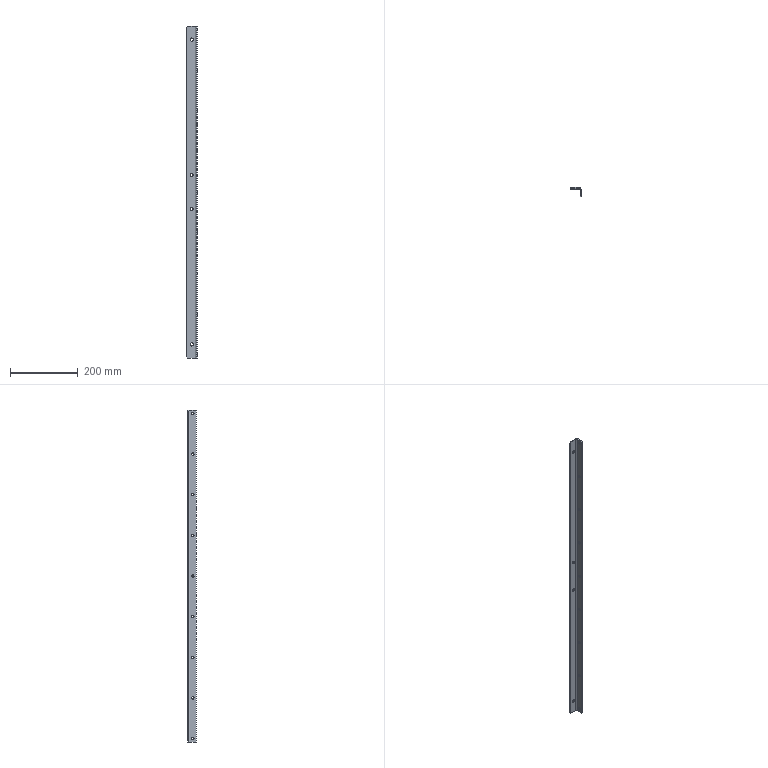Part | NX | features solid 2 | 1 solid | 38 faces | box 30 x 25 x 980 mm | volume 145338 mm3 | cylinder 28 | plane 10 | commonest cylinder face diameters 7 x18 9.2 x8 6 x1 12 x1
STEP:
#1=CARTESIAN_POINT('',(553.,497.,1245.));
#2=VERTEX_POINT('',#1);
#3=CARTESIAN_POINT('',(550.,497.,1242.));
#4=VERTEX_POINT('',#3);
#5=CARTESIAN_POINT('',(550.,497.,1242.));
#6=DIRECTION('',(-0.7071,0.,-0.7071));
#7=VECTOR('',#6,1000.);
#8=LINE('',#5,#7);
#9=EDGE_CURVE('',#2,#4,#8,.T.);
#10=ORIENTED_EDGE('',*,*,#9,.F.);
#11=CARTESIAN_POINT('',(553.,500.,1245.));
#12=VERTEX_POINT('',#11);
#13=CARTESIAN_POINT('',(553.,500.,1245.));
#14=DIRECTION('',(0.,-1.,0.));
#15=VECTOR('',#14,1000.);
#16=LINE('',#13,#15);
#17=EDGE_CURVE('',#12,#2,#16,.T.);
#18=ORIENTED_EDGE('',*,*,#17,.F.);
#19=CARTESIAN_POINT('',(550.,500.,1242.));
#20=VERTEX_POINT('',#19);
#21=CARTESIAN_POINT('',(566.5,500.,1258.5));
#22=DIRECTION('',(0.7071,0.,0.7071));
#23=VECTOR('',#22,1000.);
#24=LINE('',#21,#23);
#25=EDGE_CURVE('',#20,#12,#24,.T.);
#26=ORIENTED_EDGE('',*,*,#25,.F.);
#27=CARTESIAN_POINT('',(550.,500.,1242.));
#28=DIRECTION('',(0.,1.,0.));
#29=VECTOR('',#28,1000.);
#30=LINE('',#27,#29);
#31=EDGE_CURVE('',#4,#20,#30,.T.);
#32=ORIENTED_EDGE('',*,*,#31,.F.);
#33=EDGE_LOOP('',(#10,#18,#26,#32));
#34=FACE_BOUND('',#33,.T.);
#35=CARTESIAN_POINT('',(550.,500.,1242.));
#36=DIRECTION('',(0.7071,0.,-0.7071));
#37=DIRECTION('',(0.,-1.,0.));
#38=AXIS2_PLACEMENT_3D('',#35,#36,#37);
#39=PLANE('',#38);
#40=ADVANCED_FACE('',(#34),#39,.F.);
#41=CARTESIAN_POINT('',(550.,497.,268.));
#42=VERTEX_POINT('',#41);
#43=CARTESIAN_POINT('',(553.,497.,265.));
#44=VERTEX_POINT('',#43);
#45=CARTESIAN_POINT('',(553.,497.,265.));
#46=DIRECTION('',(0.7071,0.,-0.7071));
#47=VECTOR('',#46,1000.);
#48=LINE('',#45,#47);
#49=EDGE_CURVE('',#42,#44,#48,.T.);
#50=ORIENTED_EDGE('',*,*,#49,.F.);
#51=CARTESIAN_POINT('',(550.,500.,268.));
#52=VERTEX_POINT('',#51);
#53=CARTESIAN_POINT('',(550.,500.,268.));
#54=DIRECTION('',(0.,-1.,0.));
#55=VECTOR('',#54,1000.);
#56=LINE('',#53,#55);
#57=EDGE_CURVE('',#52,#42,#56,.T.);
#58=ORIENTED_EDGE('',*,*,#57,.F.);
#59=CARTESIAN_POINT('',(553.,500.,265.));
#60=VERTEX_POINT('',#59);
#61=CARTESIAN_POINT('',(76.5,500.,741.5));
#62=DIRECTION('',(-0.7071,0.,0.7071));
#63=VECTOR('',#62,1000.);
#64=LINE('',#61,#63);
#65=EDGE_CURVE('',#60,#52,#64,.T.);
#66=ORIENTED_EDGE('',*,*,#65,.F.);
#67=CARTESIAN_POINT('',(553.,500.,265.));
#68=DIRECTION('',(0.,1.,0.));
#69=VECTOR('',#68,1000.);
#70=LINE('',#67,#69);
#71=EDGE_CURVE('',#44,#60,#70,.T.);
#72=ORIENTED_EDGE('',*,*,#71,.F.);
#73=EDGE_LOOP('',(#50,#58,#66,#72));
#74=FACE_BOUND('',#73,.T.);
#75=CARTESIAN_POINT('',(553.,500.,265.));
#76=DIRECTION('',(-0.7071,0.,-0.7071));
#77=DIRECTION('',(-0.7071,0.,0.7071));
#78=AXIS2_PLACEMENT_3D('',#75,#76,#77);
#79=PLANE('',#78);
#80=ADVANCED_FACE('',(#74),#79,.T.);
#81=CARTESIAN_POINT('',(577.,488.5,1235.));
#82=VERTEX_POINT('',#81);
#83=CARTESIAN_POINT('',(580.,488.5,1235.));
#84=VERTEX_POINT('',#83);
#85=CARTESIAN_POINT('',(1557.778,488.5,1235.));
#86=DIRECTION('',(-1.,0.,0.));
#87=VECTOR('',#86,1000.);
#88=LINE('',#85,#87);
#89=EDGE_CURVE('',#82,#84,#88,.F.);
#90=ORIENTED_EDGE('',*,*,#89,.T.);
#91=CARTESIAN_POINT('',(580.,481.5,1235.));
#92=VERTEX_POINT('',#91);
#93=CARTESIAN_POINT('',(580.,485.,1235.));
#94=DIRECTION('',(-1.,0.,0.));
#95=DIRECTION('',(0.,-1.,0.));
#96=AXIS2_PLACEMENT_3D('',#93,#94,#95);
#97=CIRCLE('',#96,3.5);
#98=EDGE_CURVE('',#92,#84,#97,.T.);
#99=ORIENTED_EDGE('',*,*,#98,.F.);
#100=CARTESIAN_POINT('',(577.,481.5,1235.));
#101=VERTEX_POINT('',#100);
#102=CARTESIAN_POINT('',(1557.778,481.5,1235.));
#103=DIRECTION('',(-1.,0.,0.));
#104=VECTOR('',#103,1000.);
#105=LINE('',#102,#104);
#106=EDGE_CURVE('',#92,#101,#105,.T.);
#107=ORIENTED_EDGE('',*,*,#106,.T.);
#108=CARTESIAN_POINT('',(577.,485.,1235.));
#109=DIRECTION('',(-1.,0.,0.));
#110=DIRECTION('',(0.,0.,-1.));
#111=AXIS2_PLACEMENT_3D('',#108,#109,#110);
#112=CIRCLE('',#111,3.5);
#113=EDGE_CURVE('',#101,#82,#112,.T.);
#114=ORIENTED_EDGE('',*,*,#113,.T.);
#115=EDGE_LOOP('',(#90,#99,#107,#114));
#116=FACE_BOUND('',#115,.T.);
#117=CARTESIAN_POINT('',(1557.778,485.,1235.));
#118=DIRECTION('',(-1.,0.,0.));
#119=DIRECTION('',(0.,-1.,0.));
#120=AXIS2_PLACEMENT_3D('',#117,#118,#119);
#121=CYLINDRICAL_SURFACE('',#120,3.5);
#122=ADVANCED_FACE('',(#116),#121,.F.);
#123=CARTESIAN_POINT('',(580.,488.5,275.));
#124=VERTEX_POINT('',#123);
#125=CARTESIAN_POINT('',(577.,488.5,275.));
#126=VERTEX_POINT('',#125);
#127=CARTESIAN_POINT('',(1557.778,488.5,275.));
#128=DIRECTION('',(-1.,0.,0.));
#129=VECTOR('',#128,1000.);
#130=LINE('',#127,#129);
#131=EDGE_CURVE('',#124,#126,#130,.T.);
#132=ORIENTED_EDGE('',*,*,#131,.F.);
#133=CARTESIAN_POINT('',(580.,481.5,275.));
#134=VERTEX_POINT('',#133);
#135=CARTESIAN_POINT('',(580.,485.,275.));
#136=DIRECTION('',(-1.,0.,0.));
#137=DIRECTION('',(0.,-1.,0.));
#138=AXIS2_PLACEMENT_3D('',#135,#136,#137);
#139=CIRCLE('',#138,3.5);
#140=EDGE_CURVE('',#134,#124,#139,.T.);
#141=ORIENTED_EDGE('',*,*,#140,.F.);
#142=CARTESIAN_POINT('',(577.,481.5,275.));
#143=VERTEX_POINT('',#142);
#144=CARTESIAN_POINT('',(1557.778,481.5,275.));
#145=DIRECTION('',(-1.,0.,0.));
#146=VECTOR('',#145,1000.);
#147=LINE('',#144,#146);
#148=EDGE_CURVE('',#143,#134,#147,.F.);
#149=ORIENTED_EDGE('',*,*,#148,.F.);
#150=CARTESIAN_POINT('',(577.,485.,275.));
#151=DIRECTION('',(-1.,0.,0.));
#152=DIRECTION('',(0.,0.,-1.));
#153=AXIS2_PLACEMENT_3D('',#150,#151,#152);
#154=CIRCLE('',#153,3.5);
#155=EDGE_CURVE('',#143,#126,#154,.T.);
#156=ORIENTED_EDGE('',*,*,#155,.T.);
#157=EDGE_LOOP('',(#132,#141,#149,#156));
#158=FACE_BOUND('',#157,.T.);
#159=CARTESIAN_POINT('',(1557.778,485.,275.));
#160=DIRECTION('',(-1.,0.,0.));
#161=DIRECTION('',(0.,-1.,0.));
#162=AXIS2_PLACEMENT_3D('',#159,#160,#161);
#163=CYLINDRICAL_SURFACE('',#162,3.5);
#164=ADVANCED_FACE('',(#158),#163,.F.);
#165=CARTESIAN_POINT('',(580.,488.5,395.));
#166=VERTEX_POINT('',#165);
#167=CARTESIAN_POINT('',(577.,488.5,395.));
#168=VERTEX_POINT('',#167);
#169=CARTESIAN_POINT('',(1557.778,488.5,395.));
#170=DIRECTION('',(-1.,0.,0.));
#171=VECTOR('',#170,1000.);
#172=LINE('',#169,#171);
#173=EDGE_CURVE('',#166,#168,#172,.T.);
#174=ORIENTED_EDGE('',*,*,#173,.F.);
#175=CARTESIAN_POINT('',(580.,481.5,395.));
#176=VERTEX_POINT('',#175);
#177=CARTESIAN_POINT('',(580.,485.,395.));
#178=DIRECTION('',(-1.,0.,0.));
#179=DIRECTION('',(0.,-1.,0.));
#180=AXIS2_PLACEMENT_3D('',#177,#178,#179);
#181=CIRCLE('',#180,3.5);
#182=EDGE_CURVE('',#176,#166,#181,.T.);
#183=ORIENTED_EDGE('',*,*,#182,.F.);
#184=CARTESIAN_POINT('',(577.,481.5,395.));
#185=VERTEX_POINT('',#184);
#186=CARTESIAN_POINT('',(1557.778,481.5,395.));
#187=DIRECTION('',(-1.,0.,0.));
#188=VECTOR('',#187,1000.);
#189=LINE('',#186,#188);
#190=EDGE_CURVE('',#185,#176,#189,.F.);
#191=ORIENTED_EDGE('',*,*,#190,.F.);
#192=CARTESIAN_POINT('',(577.,485.,395.));
#193=DIRECTION('',(-1.,0.,0.));
#194=DIRECTION('',(0.,0.,-1.));
#195=AXIS2_PLACEMENT_3D('',#192,#193,#194);
#196=CIRCLE('',#195,3.5);
#197=EDGE_CURVE('',#185,#168,#196,.T.);
#198=ORIENTED_EDGE('',*,*,#197,.T.);
#199=EDGE_LOOP('',(#174,#183,#191,#198));
#200=FACE_BOUND('',#199,.T.);
#201=CARTESIAN_POINT('',(1557.778,485.,395.));
#202=DIRECTION('',(-1.,0.,0.));
#203=DIRECTION('',(0.,-1.,0.));
#204=AXIS2_PLACEMENT_3D('',#201,#202,#203);
#205=CYLINDRICAL_SURFACE('',#204,3.5);
#206=ADVANCED_FACE('',(#200),#205,.F.);
#207=CARTESIAN_POINT('',(577.,488.5,1115.));
#208=VERTEX_POINT('',#207);
#209=CARTESIAN_POINT('',(580.,488.5,1115.));
#210=VERTEX_POINT('',#209);
#211=CARTESIAN_POINT('',(1557.778,488.5,1115.));
#212=DIRECTION('',(-1.,0.,0.));
#213=VECTOR('',#212,1000.);
#214=LINE('',#211,#213);
#215=EDGE_CURVE('',#208,#210,#214,.F.);
#216=ORIENTED_EDGE('',*,*,#215,.T.);
#217=CARTESIAN_POINT('',(580.,481.5,1115.));
#218=VERTEX_POINT('',#217);
#219=CARTESIAN_POINT('',(580.,485.,1115.));
#220=DIRECTION('',(-1.,0.,0.));
#221=DIRECTION('',(0.,-1.,0.));
#222=AXIS2_PLACEMENT_3D('',#219,#220,#221);
#223=CIRCLE('',#222,3.5);
#224=EDGE_CURVE('',#218,#210,#223,.T.);
#225=ORIENTED_EDGE('',*,*,#224,.F.);
#226=CARTESIAN_POINT('',(577.,481.5,1115.));
#227=VERTEX_POINT('',#226);
#228=CARTESIAN_POINT('',(1557.778,481.5,1115.));
#229=DIRECTION('',(-1.,0.,0.));
#230=VECTOR('',#229,1000.);
#231=LINE('',#228,#230);
#232=EDGE_CURVE('',#218,#227,#231,.T.);
#233=ORIENTED_EDGE('',*,*,#232,.T.);
#234=CARTESIAN_POINT('',(577.,485.,1115.));
#235=DIRECTION('',(-1.,0.,0.));
#236=DIRECTION('',(0.,0.,-1.));
#237=AXIS2_PLACEMENT_3D('',#234,#235,#236);
#238=CIRCLE('',#237,3.5);
#239=EDGE_CURVE('',#227,#208,#238,.T.);
#240=ORIENTED_EDGE('',*,*,#239,.T.);
#241=EDGE_LOOP('',(#216,#225,#233,#240));
#242=FACE_BOUND('',#241,.T.);
#243=CARTESIAN_POINT('',(1557.778,485.,1115.));
#244=DIRECTION('',(-1.,0.,0.));
#245=DIRECTION('',(0.,-1.,0.));
#246=AXIS2_PLACEMENT_3D('',#243,#244,#245);
#247=CYLINDRICAL_SURFACE('',#246,3.5);
#248=ADVANCED_FACE('',(#242),#247,.F.);
#249=CARTESIAN_POINT('',(577.,488.5,995.));
#250=VERTEX_POINT('',#249);
#251=CARTESIAN_POINT('',(580.,488.5,995.));
#252=VERTEX_POINT('',#251);
#253=CARTESIAN_POINT('',(1557.778,488.5,995.));
#254=DIRECTION('',(-1.,0.,0.));
#255=VECTOR('',#254,1000.);
#256=LINE('',#253,#255);
#257=EDGE_CURVE('',#250,#252,#256,.F.);
#258=ORIENTED_EDGE('',*,*,#257,.T.);
#259=CARTESIAN_POINT('',(580.,481.5,995.));
#260=VERTEX_POINT('',#259);
#261=CARTESIAN_POINT('',(580.,485.,995.));
#262=DIRECTION('',(-1.,0.,0.));
#263=DIRECTION('',(0.,-1.,0.));
#264=AXIS2_PLACEMENT_3D('',#261,#262,#263);
#265=CIRCLE('',#264,3.5);
#266=EDGE_CURVE('',#260,#252,#265,.T.);
#267=ORIENTED_EDGE('',*,*,#266,.F.);
#268=CARTESIAN_POINT('',(577.,481.5,995.));
#269=VERTEX_POINT('',#268);
#270=CARTESIAN_POINT('',(1557.778,481.5,995.));
#271=DIRECTION('',(-1.,0.,0.));
#272=VECTOR('',#271,1000.);
#273=LINE('',#270,#272);
#274=EDGE_CURVE('',#260,#269,#273,.T.);
#275=ORIENTED_EDGE('',*,*,#274,.T.);
#276=CARTESIAN_POINT('',(577.,485.,995.));
#277=DIRECTION('',(-1.,0.,0.));
#278=DIRECTION('',(0.,0.,-1.));
#279=AXIS2_PLACEMENT_3D('',#276,#277,#278);
#280=CIRCLE('',#279,3.5);
#281=EDGE_CURVE('',#269,#250,#280,.T.);
#282=ORIENTED_EDGE('',*,*,#281,.T.);
#283=EDGE_LOOP('',(#258,#267,#275,#282));
#284=FACE_BOUND('',#283,.T.);
#285=CARTESIAN_POINT('',(1557.778,485.,995.));
#286=DIRECTION('',(-1.,0.,0.));
#287=DIRECTION('',(0.,-1.,0.));
#288=AXIS2_PLACEMENT_3D('',#285,#286,#287);
#289=CYLINDRICAL_SURFACE('',#288,3.5);
#290=ADVANCED_FACE('',(#284),#289,.F.);
#291=CARTESIAN_POINT('',(580.,488.5,875.));
#292=VERTEX_POINT('',#291);
#293=CARTESIAN_POINT('',(577.,488.5,875.));
#294=VERTEX_POINT('',#293);
#295=CARTESIAN_POINT('',(1557.778,488.5,875.));
#296=DIRECTION('',(-1.,0.,0.));
#297=VECTOR('',#296,1000.);
#298=LINE('',#295,#297);
#299=EDGE_CURVE('',#292,#294,#298,.T.);
#300=ORIENTED_EDGE('',*,*,#299,.F.);
#301=CARTESIAN_POINT('',(580.,481.5,875.));
#302=VERTEX_POINT('',#301);
#303=CARTESIAN_POINT('',(580.,485.,875.));
#304=DIRECTION('',(-1.,0.,0.));
#305=DIRECTION('',(0.,-1.,0.));
#306=AXIS2_PLACEMENT_3D('',#303,#304,#305);
#307=CIRCLE('',#306,3.5);
#308=EDGE_CURVE('',#302,#292,#307,.T.);
#309=ORIENTED_EDGE('',*,*,#308,.F.);
#310=CARTESIAN_POINT('',(577.,481.5,875.));
#311=VERTEX_POINT('',#310);
#312=CARTESIAN_POINT('',(1557.778,481.5,875.));
#313=DIRECTION('',(-1.,0.,0.));
#314=VECTOR('',#313,1000.);
#315=LINE('',#312,#314);
#316=EDGE_CURVE('',#311,#302,#315,.F.);
#317=ORIENTED_EDGE('',*,*,#316,.F.);
#318=CARTESIAN_POINT('',(577.,485.,875.));
#319=DIRECTION('',(-1.,0.,0.));
#320=DIRECTION('',(0.,0.,-1.));
#321=AXIS2_PLACEMENT_3D('',#318,#319,#320);
#322=CIRCLE('',#321,3.5);
#323=EDGE_CURVE('',#311,#294,#322,.T.);
#324=ORIENTED_EDGE('',*,*,#323,.T.);
#325=EDGE_LOOP('',(#300,#309,#317,#324));
#326=FACE_BOUND('',#325,.T.);
#327=CARTESIAN_POINT('',(1557.778,485.,875.));
#328=DIRECTION('',(-1.,0.,0.));
#329=DIRECTION('',(0.,-1.,0.));
#330=AXIS2_PLACEMENT_3D('',#327,#328,#329);
#331=CYLINDRICAL_SURFACE('',#330,3.5);
#332=ADVANCED_FACE('',(#326),#331,.F.);
#333=CARTESIAN_POINT('',(580.,488.5,755.));
#334=VERTEX_POINT('',#333);
#335=CARTESIAN_POINT('',(577.,488.5,755.));
#336=VERTEX_POINT('',#335);
#337=CARTESIAN_POINT('',(1557.778,488.5,755.));
#338=DIRECTION('',(-1.,0.,0.));
#339=VECTOR('',#338,1000.);
#340=LINE('',#337,#339);
#341=EDGE_CURVE('',#334,#336,#340,.T.);
#342=ORIENTED_EDGE('',*,*,#341,.F.);
#343=CARTESIAN_POINT('',(580.,481.5,755.));
#344=VERTEX_POINT('',#343);
#345=CARTESIAN_POINT('',(580.,485.,755.));
#346=DIRECTION('',(-1.,0.,0.));
#347=DIRECTION('',(0.,-1.,0.));
#348=AXIS2_PLACEMENT_3D('',#345,#346,#347);
#349=CIRCLE('',#348,3.5);
#350=EDGE_CURVE('',#344,#334,#349,.T.);
#351=ORIENTED_EDGE('',*,*,#350,.F.);
#352=CARTESIAN_POINT('',(577.,481.5,755.));
#353=VERTEX_POINT('',#352);
#354=CARTESIAN_POINT('',(1557.778,481.5,755.));
#355=DIRECTION('',(-1.,0.,0.));
#356=VECTOR('',#355,1000.);
#357=LINE('',#354,#356);
#358=EDGE_CURVE('',#353,#344,#357,.F.);
#359=ORIENTED_EDGE('',*,*,#358,.F.);
#360=CARTESIAN_POINT('',(577.,485.,755.));
#361=DIRECTION('',(-1.,0.,0.));
#362=DIRECTION('',(0.,0.,-1.));
#363=AXIS2_PLACEMENT_3D('',#360,#361,#362);
#364=CIRCLE('',#363,3.5);
#365=EDGE_CURVE('',#353,#336,#364,.T.);
#366=ORIENTED_EDGE('',*,*,#365,.T.);
#367=EDGE_LOOP('',(#342,#351,#359,#366));
#368=FACE_BOUND('',#367,.T.);
#369=CARTESIAN_POINT('',(1557.778,485.,755.));
#370=DIRECTION('',(-1.,0.,0.));
#371=DIRECTION('',(0.,-1.,0.));
#372=AXIS2_PLACEMENT_3D('',#369,#370,#371);
#373=CYLINDRICAL_SURFACE('',#372,3.5);
#374=ADVANCED_FACE('',(#368),#373,.F.);
#375=CARTESIAN_POINT('',(577.,488.5,635.));
#376=VERTEX_POINT('',#375);
#377=CARTESIAN_POINT('',(580.,488.5,635.));
#378=VERTEX_POINT('',#377);
#379=CARTESIAN_POINT('',(1557.778,488.5,635.));
#380=DIRECTION('',(-1.,0.,0.));
#381=VECTOR('',#380,1000.);
#382=LINE('',#379,#381);
#383=EDGE_CURVE('',#376,#378,#382,.F.);
#384=ORIENTED_EDGE('',*,*,#383,.T.);
#385=CARTESIAN_POINT('',(580.,481.5,635.));
#386=VERTEX_POINT('',#385);
#387=CARTESIAN_POINT('',(580.,485.,635.));
#388=DIRECTION('',(-1.,0.,0.));
#389=DIRECTION('',(0.,-1.,0.));
#390=AXIS2_PLACEMENT_3D('',#387,#388,#389);
#391=CIRCLE('',#390,3.5);
#392=EDGE_CURVE('',#386,#378,#391,.T.);
#393=ORIENTED_EDGE('',*,*,#392,.F.);
#394=CARTESIAN_POINT('',(577.,481.5,635.));
#395=VERTEX_POINT('',#394);
#396=CARTESIAN_POINT('',(1557.778,481.5,635.));
#397=DIRECTION('',(-1.,0.,0.));
#398=VECTOR('',#397,1000.);
#399=LINE('',#396,#398);
#400=EDGE_CURVE('',#386,#395,#399,.T.);
#401=ORIENTED_EDGE('',*,*,#400,.T.);
#402=CARTESIAN_POINT('',(577.,485.,635.));
#403=DIRECTION('',(-1.,0.,0.));
#404=DIRECTION('',(0.,0.,-1.));
#405=AXIS2_PLACEMENT_3D('',#402,#403,#404);
#406=CIRCLE('',#405,3.5);
#407=EDGE_CURVE('',#395,#376,#406,.T.);
#408=ORIENTED_EDGE('',*,*,#407,.T.);
#409=EDGE_LOOP('',(#384,#393,#401,#408));
#410=FACE_BOUND('',#409,.T.);
#411=CARTESIAN_POINT('',(1557.778,485.,635.));
#412=DIRECTION('',(-1.,0.,0.));
#413=DIRECTION('',(0.,-1.,0.));
#414=AXIS2_PLACEMENT_3D('',#411,#412,#413);
#415=CYLINDRICAL_SURFACE('',#414,3.5);
#416=ADVANCED_FACE('',(#410),#415,.F.);
#417=CARTESIAN_POINT('',(580.,488.5,515.));
#418=VERTEX_POINT('',#417);
#419=CARTESIAN_POINT('',(577.,488.5,515.));
#420=VERTEX_POINT('',#419);
#421=CARTESIAN_POINT('',(1557.778,488.5,515.));
#422=DIRECTION('',(-1.,0.,0.));
#423=VECTOR('',#422,1000.);
#424=LINE('',#421,#423);
#425=EDGE_CURVE('',#418,#420,#424,.T.);
#426=ORIENTED_EDGE('',*,*,#425,.F.);
#427=CARTESIAN_POINT('',(580.,481.5,515.));
#428=VERTEX_POINT('',#427);
#429=CARTESIAN_POINT('',(580.,485.,515.));
#430=DIRECTION('',(-1.,0.,0.));
#431=DIRECTION('',(0.,-1.,0.));
#432=AXIS2_PLACEMENT_3D('',#429,#430,#431);
#433=CIRCLE('',#432,3.5);
#434=EDGE_CURVE('',#428,#418,#433,.T.);
#435=ORIENTED_EDGE('',*,*,#434,.F.);
#436=CARTESIAN_POINT('',(577.,481.5,515.));
#437=VERTEX_POINT('',#436);
#438=CARTESIAN_POINT('',(1557.778,481.5,515.));
#439=DIRECTION('',(-1.,0.,0.));
#440=VECTOR('',#439,1000.);
#441=LINE('',#438,#440);
#442=EDGE_CURVE('',#437,#428,#441,.F.);
#443=ORIENTED_EDGE('',*,*,#442,.F.);
#444=CARTESIAN_POINT('',(577.,485.,515.));
#445=DIRECTION('',(-1.,0.,0.));
#446=DIRECTION('',(0.,0.,-1.));
#447=AXIS2_PLACEMENT_3D('',#444,#445,#446);
#448=CIRCLE('',#447,3.5);
#449=EDGE_CURVE('',#437,#420,#448,.T.);
#450=ORIENTED_EDGE('',*,*,#449,.T.);
#451=EDGE_LOOP('',(#426,#435,#443,#450));
#452=FACE_BOUND('',#451,.T.);
#453=CARTESIAN_POINT('',(1557.778,485.,515.));
#454=DIRECTION('',(-1.,0.,0.));
#455=DIRECTION('',(0.,-1.,0.));
#456=AXIS2_PLACEMENT_3D('',#453,#454,#455);
#457=CYLINDRICAL_SURFACE('',#456,3.5);
#458=ADVANCED_FACE('',(#452),#457,.F.);
#459=CARTESIAN_POINT('',(564.,500.,1209.6));
#460=VERTEX_POINT('',#459);
#461=CARTESIAN_POINT('',(564.,497.,1209.6));
#462=VERTEX_POINT('',#461);
#463=CARTESIAN_POINT('',(564.,-480.778,1209.6));
#464=DIRECTION('',(0.,1.,0.));
#465=VECTOR('',#464,1000.);
#466=LINE('',#463,#465);
#467=EDGE_CURVE('',#460,#462,#466,.F.);
#468=ORIENTED_EDGE('',*,*,#467,.T.);
#469=CARTESIAN_POINT('',(564.,497.,1200.4));
#470=VERTEX_POINT('',#469);
#471=CARTESIAN_POINT('',(564.,497.,1205.));
#472=DIRECTION('',(0.,1.,0.));
#473=DIRECTION('',(0.,0.,-1.));
#474=AXIS2_PLACEMENT_3D('',#471,#472,#473);
#475=CIRCLE('',#474,4.6);
#476=EDGE_CURVE('',#470,#462,#475,.T.);
#477=ORIENTED_EDGE('',*,*,#476,.F.);
#478=CARTESIAN_POINT('',(564.,500.,1200.4));
#479=VERTEX_POINT('',#478);
#480=CARTESIAN_POINT('',(564.,-480.778,1200.4));
#481=DIRECTION('',(0.,1.,0.));
#482=VECTOR('',#481,1000.);
#483=LINE('',#480,#482);
#484=EDGE_CURVE('',#470,#479,#483,.T.);
#485=ORIENTED_EDGE('',*,*,#484,.T.);
#486=CARTESIAN_POINT('',(564.,500.,1205.));
#487=DIRECTION('',(0.,1.,0.));
#488=DIRECTION('',(0.,0.,1.));
#489=AXIS2_PLACEMENT_3D('',#486,#487,#488);
#490=CIRCLE('',#489,4.6);
#491=EDGE_CURVE('',#479,#460,#490,.T.);
#492=ORIENTED_EDGE('',*,*,#491,.T.);
#493=EDGE_LOOP('',(#468,#477,#485,#492));
#494=FACE_BOUND('',#493,.T.);
#495=CARTESIAN_POINT('',(564.,-480.778,1205.));
#496=DIRECTION('',(0.,1.,0.));
#497=DIRECTION('',(0.,0.,-1.));
#498=AXIS2_PLACEMENT_3D('',#495,#496,#497);
#499=CYLINDRICAL_SURFACE('',#498,4.6);
#500=ADVANCED_FACE('',(#494),#499,.F.);
#501=CARTESIAN_POINT('',(564.,497.,709.6));
#502=VERTEX_POINT('',#501);
#503=CARTESIAN_POINT('',(564.,500.,709.6));
#504=VERTEX_POINT('',#503);
#505=CARTESIAN_POINT('',(564.,-480.778,709.6));
#506=DIRECTION('',(0.,1.,0.));
#507=VECTOR('',#506,1000.);
#508=LINE('',#505,#507);
#509=EDGE_CURVE('',#502,#504,#508,.T.);
#510=ORIENTED_EDGE('',*,*,#509,.F.);
#511=CARTESIAN_POINT('',(564.,497.,700.4));
#512=VERTEX_POINT('',#511);
#513=CARTESIAN_POINT('',(564.,497.,705.));
#514=DIRECTION('',(0.,1.,0.));
#515=DIRECTION('',(0.,0.,-1.));
#516=AXIS2_PLACEMENT_3D('',#513,#514,#515);
#517=CIRCLE('',#516,4.6);
#518=EDGE_CURVE('',#512,#502,#517,.T.);
#519=ORIENTED_EDGE('',*,*,#518,.F.);
#520=CARTESIAN_POINT('',(564.,500.,700.4));
#521=VERTEX_POINT('',#520);
#522=CARTESIAN_POINT('',(564.,-480.778,700.4));
#523=DIRECTION('',(0.,1.,0.));
#524=VECTOR('',#523,1000.);
#525=LINE('',#522,#524);
#526=EDGE_CURVE('',#521,#512,#525,.F.);
#527=ORIENTED_EDGE('',*,*,#526,.F.);
#528=CARTESIAN_POINT('',(564.,500.,705.));
#529=DIRECTION('',(0.,1.,0.));
#530=DIRECTION('',(0.,0.,1.));
#531=AXIS2_PLACEMENT_3D('',#528,#529,#530);
#532=CIRCLE('',#531,4.6);
#533=EDGE_CURVE('',#521,#504,#532,.T.);
#534=ORIENTED_EDGE('',*,*,#533,.T.);
#535=EDGE_LOOP('',(#510,#519,#527,#534));
#536=FACE_BOUND('',#535,.T.);
#537=CARTESIAN_POINT('',(564.,-480.778,705.));
#538=DIRECTION('',(0.,1.,0.));
#539=DIRECTION('',(0.,0.,-1.));
#540=AXIS2_PLACEMENT_3D('',#537,#538,#539);
#541=CYLINDRICAL_SURFACE('',#540,4.6);
#542=ADVANCED_FACE('',(#536),#541,.F.);
#543=CARTESIAN_POINT('',(564.,500.,809.6));
#544=VERTEX_POINT('',#543);
#545=CARTESIAN_POINT('',(564.,497.,809.6));
#546=VERTEX_POINT('',#545);
#547=CARTESIAN_POINT('',(564.,-480.778,809.6));
#548=DIRECTION('',(0.,1.,0.));
#549=VECTOR('',#548,1000.);
#550=LINE('',#547,#549);
#551=EDGE_CURVE('',#544,#546,#550,.F.);
#552=ORIENTED_EDGE('',*,*,#551,.T.);
#553=CARTESIAN_POINT('',(564.,497.,800.4));
#554=VERTEX_POINT('',#553);
#555=CARTESIAN_POINT('',(564.,497.,805.));
#556=DIRECTION('',(0.,1.,0.));
#557=DIRECTION('',(0.,0.,-1.));
#558=AXIS2_PLACEMENT_3D('',#555,#556,#557);
#559=CIRCLE('',#558,4.6);
#560=EDGE_CURVE('',#554,#546,#559,.T.);
#561=ORIENTED_EDGE('',*,*,#560,.F.);
#562=CARTESIAN_POINT('',(564.,500.,800.4));
#563=VERTEX_POINT('',#562);
#564=CARTESIAN_POINT('',(564.,-480.778,800.4));
#565=DIRECTION('',(0.,1.,0.));
#566=VECTOR('',#565,1000.);
#567=LINE('',#564,#566);
#568=EDGE_CURVE('',#554,#563,#567,.T.);
#569=ORIENTED_EDGE('',*,*,#568,.T.);
#570=CARTESIAN_POINT('',(564.,500.,805.));
#571=DIRECTION('',(0.,1.,0.));
#572=DIRECTION('',(0.,0.,1.));
#573=AXIS2_PLACEMENT_3D('',#570,#571,#572);
#574=CIRCLE('',#573,4.6);
#575=EDGE_CURVE('',#563,#544,#574,.T.);
#576=ORIENTED_EDGE('',*,*,#575,.T.);
#577=EDGE_LOOP('',(#552,#561,#569,#576));
#578=FACE_BOUND('',#577,.T.);
#579=CARTESIAN_POINT('',(564.,-480.778,805.));
#580=DIRECTION('',(0.,1.,0.));
#581=DIRECTION('',(0.,0.,-1.));
#582=AXIS2_PLACEMENT_3D('',#579,#580,#581);
#583=CYLINDRICAL_SURFACE('',#582,4.6);
#584=ADVANCED_FACE('',(#578),#583,.F.);
#585=CARTESIAN_POINT('',(564.,500.,309.6));
#586=VERTEX_POINT('',#585);
#587=CARTESIAN_POINT('',(564.,497.,309.6));
#588=VERTEX_POINT('',#587);
#589=CARTESIAN_POINT('',(564.,-480.778,309.6));
#590=DIRECTION('',(0.,1.,0.));
#591=VECTOR('',#590,1000.);
#592=LINE('',#589,#591);
#593=EDGE_CURVE('',#586,#588,#592,.F.);
#594=ORIENTED_EDGE('',*,*,#593,.T.);
#595=CARTESIAN_POINT('',(564.,497.,300.4));
#596=VERTEX_POINT('',#595);
#597=CARTESIAN_POINT('',(564.,497.,305.));
#598=DIRECTION('',(0.,1.,0.));
#599=DIRECTION('',(0.,0.,-1.));
#600=AXIS2_PLACEMENT_3D('',#597,#598,#599);
#601=CIRCLE('',#600,4.6);
#602=EDGE_CURVE('',#596,#588,#601,.T.);
#603=ORIENTED_EDGE('',*,*,#602,.F.);
#604=CARTESIAN_POINT('',(564.,500.,300.4));
#605=VERTEX_POINT('',#604);
#606=CARTESIAN_POINT('',(564.,-480.778,300.4));
#607=DIRECTION('',(0.,1.,0.));
#608=VECTOR('',#607,1000.);
#609=LINE('',#606,#608);
#610=EDGE_CURVE('',#596,#605,#609,.T.);
#611=ORIENTED_EDGE('',*,*,#610,.T.);
#612=CARTESIAN_POINT('',(564.,500.,305.));
#613=DIRECTION('',(0.,1.,0.));
#614=DIRECTION('',(0.,0.,1.));
#615=AXIS2_PLACEMENT_3D('',#612,#613,#614);
#616=CIRCLE('',#615,4.6);
#617=EDGE_CURVE('',#605,#586,#616,.T.);
#618=ORIENTED_EDGE('',*,*,#617,.T.);
#619=EDGE_LOOP('',(#594,#603,#611,#618));
#620=FACE_BOUND('',#619,.T.);
#621=CARTESIAN_POINT('',(564.,-480.778,305.));
#622=DIRECTION('',(0.,1.,0.));
#623=DIRECTION('',(0.,0.,-1.));
#624=AXIS2_PLACEMENT_3D('',#621,#622,#623);
#625=CYLINDRICAL_SURFACE('',#624,4.6);
#626=ADVANCED_FACE('',(#620),#625,.F.);
#627=CARTESIAN_POINT('',(574.,497.,1245.));
#628=VERTEX_POINT('',#627);
#629=CARTESIAN_POINT('',(574.,497.,265.));
#630=VERTEX_POINT('',#629);
#631=CARTESIAN_POINT('',(574.,497.,1245.));
#632=DIRECTION('',(0.,0.,-1.));
#633=VECTOR('',#632,1000.);
#634=LINE('',#631,#633);
#635=EDGE_CURVE('',#628,#630,#634,.T.);
#636=ORIENTED_EDGE('',*,*,#635,.T.);
#637=CARTESIAN_POINT('',(577.,494.,265.));
#638=VERTEX_POINT('',#637);
#639=CARTESIAN_POINT('',(574.,494.,265.));
#640=DIRECTION('',(0.,0.,1.));
#641=DIRECTION('',(0.,-1.,0.));
#642=AXIS2_PLACEMENT_3D('',#639,#640,#641);
#643=CIRCLE('',#642,3.);
#644=EDGE_CURVE('',#638,#630,#643,.T.);
#645=ORIENTED_EDGE('',*,*,#644,.F.);
#646=CARTESIAN_POINT('',(577.,494.,1245.));
#647=VERTEX_POINT('',#646);
#648=CARTESIAN_POINT('',(577.,494.,265.));
#649=DIRECTION('',(0.,0.,1.));
#650=VECTOR('',#649,1000.);
#651=LINE('',#648,#650);
#652=EDGE_CURVE('',#638,#647,#651,.T.);
#653=ORIENTED_EDGE('',*,*,#652,.T.);
#654=CARTESIAN_POINT('',(574.,494.,1245.));
#655=DIRECTION('',(0.,0.,1.));
#656=DIRECTION('',(0.,-1.,0.));
#657=AXIS2_PLACEMENT_3D('',#654,#655,#656);
#658=CIRCLE('',#657,3.);
#659=EDGE_CURVE('',#647,#628,#658,.T.);
#660=ORIENTED_EDGE('',*,*,#659,.T.);
#661=EDGE_LOOP('',(#636,#645,#653,#660));
#662=FACE_BOUND('',#661,.T.);
#663=CARTESIAN_POINT('',(574.,494.,1245.));
#664=DIRECTION('',(0.,0.,-1.));
#665=DIRECTION('',(0.,-1.,0.));
#666=AXIS2_PLACEMENT_3D('',#663,#664,#665);
#667=CYLINDRICAL_SURFACE('',#666,3.);
#668=ADVANCED_FACE('',(#662),#667,.F.);
#669=CARTESIAN_POINT('',(574.,500.,1245.));
#670=VERTEX_POINT('',#669);
#671=CARTESIAN_POINT('',(574.,500.,265.));
#672=VERTEX_POINT('',#671);
#673=CARTESIAN_POINT('',(574.,500.,1245.));
#674=DIRECTION('',(0.,0.,-1.));
#675=VECTOR('',#674,1000.);
#676=LINE('',#673,#675);
#677=EDGE_CURVE('',#670,#672,#676,.T.);
#678=ORIENTED_EDGE('',*,*,#677,.F.);
#679=CARTESIAN_POINT('',(580.,494.,1245.));
#680=VERTEX_POINT('',#679);
#681=CARTESIAN_POINT('',(574.,494.,1245.));
#682=DIRECTION('',(0.,0.,1.));
#683=DIRECTION('',(0.,-1.,0.));
#684=AXIS2_PLACEMENT_3D('',#681,#682,#683);
#685=CIRCLE('',#684,6.);
#686=EDGE_CURVE('',#680,#670,#685,.T.);
#687=ORIENTED_EDGE('',*,*,#686,.F.);
#688=CARTESIAN_POINT('',(580.,494.,265.));
#689=VERTEX_POINT('',#688);
#690=CARTESIAN_POINT('',(580.,494.,265.));
#691=DIRECTION('',(0.,0.,1.));
#692=VECTOR('',#691,1000.);
#693=LINE('',#690,#692);
#694=EDGE_CURVE('',#689,#680,#693,.T.);
#695=ORIENTED_EDGE('',*,*,#694,.F.);
#696=CARTESIAN_POINT('',(574.,494.,265.));
#697=DIRECTION('',(0.,0.,1.));
#698=DIRECTION('',(0.,-1.,0.));
#699=AXIS2_PLACEMENT_3D('',#696,#697,#698);
#700=CIRCLE('',#699,6.);
#701=EDGE_CURVE('',#689,#672,#700,.T.);
#702=ORIENTED_EDGE('',*,*,#701,.T.);
#703=EDGE_LOOP('',(#678,#687,#695,#702));
#704=FACE_BOUND('',#703,.T.);
#705=CARTESIAN_POINT('',(574.,494.,1245.));
#706=DIRECTION('',(0.,0.,-1.));
#707=DIRECTION('',(0.,-1.,0.));
#708=AXIS2_PLACEMENT_3D('',#705,#706,#707);
#709=CYLINDRICAL_SURFACE('',#708,6.);
#710=ADVANCED_FACE('',(#704),#709,.T.);
#711=ORIENTED_EDGE('',*,*,#449,.F.);
#712=CARTESIAN_POINT('',(577.,485.,515.));
#713=DIRECTION('',(-1.,0.,0.));
#714=DIRECTION('',(0.,0.,-1.));
#715=AXIS2_PLACEMENT_3D('',#712,#713,#714);
#716=CIRCLE('',#715,3.5);
#717=EDGE_CURVE('',#420,#437,#716,.T.);
#718=ORIENTED_EDGE('',*,*,#717,.F.);
#719=EDGE_LOOP('',(#711,#718));
#720=FACE_BOUND('',#719,.T.);
#721=ORIENTED_EDGE('',*,*,#407,.F.);
#722=CARTESIAN_POINT('',(577.,485.,635.));
#723=DIRECTION('',(-1.,0.,0.));
#724=DIRECTION('',(0.,0.,-1.));
#725=AXIS2_PLACEMENT_3D('',#722,#723,#724);
#726=CIRCLE('',#725,3.5);
#727=EDGE_CURVE('',#376,#395,#726,.T.);
#728=ORIENTED_EDGE('',*,*,#727,.F.);
#729=EDGE_LOOP('',(#721,#728));
#730=FACE_BOUND('',#729,.T.);
#731=ORIENTED_EDGE('',*,*,#365,.F.);
#732=CARTESIAN_POINT('',(577.,485.,755.));
#733=DIRECTION('',(-1.,0.,0.));
#734=DIRECTION('',(0.,0.,-1.));
#735=AXIS2_PLACEMENT_3D('',#732,#733,#734);
#736=CIRCLE('',#735,3.5);
#737=EDGE_CURVE('',#336,#353,#736,.T.);
#738=ORIENTED_EDGE('',*,*,#737,.F.);
#739=EDGE_LOOP('',(#731,#738));
#740=FACE_BOUND('',#739,.T.);
#741=ORIENTED_EDGE('',*,*,#323,.F.);
#742=CARTESIAN_POINT('',(577.,485.,875.));
#743=DIRECTION('',(-1.,0.,0.));
#744=DIRECTION('',(0.,0.,-1.));
#745=AXIS2_PLACEMENT_3D('',#742,#743,#744);
#746=CIRCLE('',#745,3.5);
#747=EDGE_CURVE('',#294,#311,#746,.T.);
#748=ORIENTED_EDGE('',*,*,#747,.F.);
#749=EDGE_LOOP('',(#741,#748));
#750=FACE_BOUND('',#749,.T.);
#751=ORIENTED_EDGE('',*,*,#281,.F.);
#752=CARTESIAN_POINT('',(577.,485.,995.));
#753=DIRECTION('',(-1.,0.,0.));
#754=DIRECTION('',(0.,0.,-1.));
#755=AXIS2_PLACEMENT_3D('',#752,#753,#754);
#756=CIRCLE('',#755,3.5);
#757=EDGE_CURVE('',#250,#269,#756,.T.);
#758=ORIENTED_EDGE('',*,*,#757,.F.);
#759=EDGE_LOOP('',(#751,#758));
#760=FACE_BOUND('',#759,.T.);
#761=ORIENTED_EDGE('',*,*,#239,.F.);
#762=CARTESIAN_POINT('',(577.,485.,1115.));
#763=DIRECTION('',(-1.,0.,0.));
#764=DIRECTION('',(0.,0.,-1.));
#765=AXIS2_PLACEMENT_3D('',#762,#763,#764);
#766=CIRCLE('',#765,3.5);
#767=EDGE_CURVE('',#208,#227,#766,.T.);
#768=ORIENTED_EDGE('',*,*,#767,.F.);
#769=EDGE_LOOP('',(#761,#768));
#770=FACE_BOUND('',#769,.T.);
#771=ORIENTED_EDGE('',*,*,#197,.F.);
#772=CARTESIAN_POINT('',(577.,485.,395.));
#773=DIRECTION('',(-1.,0.,0.));
#774=DIRECTION('',(0.,0.,-1.));
#775=AXIS2_PLACEMENT_3D('',#772,#773,#774);
#776=CIRCLE('',#775,3.5);
#777=EDGE_CURVE('',#168,#185,#776,.T.);
#778=ORIENTED_EDGE('',*,*,#777,.F.);
#779=EDGE_LOOP('',(#771,#778));
#780=FACE_BOUND('',#779,.T.);
#781=ORIENTED_EDGE('',*,*,#155,.F.);
#782=CARTESIAN_POINT('',(577.,485.,275.));
#783=DIRECTION('',(-1.,0.,0.));
#784=DIRECTION('',(0.,0.,-1.));
#785=AXIS2_PLACEMENT_3D('',#782,#783,#784);
#786=CIRCLE('',#785,3.5);
#787=EDGE_CURVE('',#126,#143,#786,.T.);
#788=ORIENTED_EDGE('',*,*,#787,.F.);
#789=EDGE_LOOP('',(#781,#788));
#790=FACE_BOUND('',#789,.T.);
#791=ORIENTED_EDGE('',*,*,#113,.F.);
#792=CARTESIAN_POINT('',(577.,485.,1235.));
#793=DIRECTION('',(-1.,0.,0.));
#794=DIRECTION('',(0.,0.,-1.));
#795=AXIS2_PLACEMENT_3D('',#792,#793,#794);
#796=CIRCLE('',#795,3.5);
#797=EDGE_CURVE('',#82,#101,#796,.T.);
#798=ORIENTED_EDGE('',*,*,#797,.F.);
#799=EDGE_LOOP('',(#791,#798));
#800=FACE_BOUND('',#799,.T.);
#801=CARTESIAN_POINT('',(577.,475.,1245.));
#802=VERTEX_POINT('',#801);
#803=CARTESIAN_POINT('',(577.,500.,1245.));
#804=DIRECTION('',(0.,-1.,0.));
#805=VECTOR('',#804,1000.);
#806=LINE('',#803,#805);
#807=EDGE_CURVE('',#647,#802,#806,.T.);
#808=ORIENTED_EDGE('',*,*,#807,.F.);
#809=ORIENTED_EDGE('',*,*,#652,.F.);
#810=CARTESIAN_POINT('',(577.,475.,265.));
#811=VERTEX_POINT('',#810);
#812=CARTESIAN_POINT('',(577.,500.,265.));
#813=DIRECTION('',(0.,-1.,0.));
#814=VECTOR('',#813,1000.);
#815=LINE('',#812,#814);
#816=EDGE_CURVE('',#638,#811,#815,.T.);
#817=ORIENTED_EDGE('',*,*,#816,.T.);
#818=CARTESIAN_POINT('',(577.,475.,265.));
#819=DIRECTION('',(0.,0.,1.));
#820=VECTOR('',#819,1000.);
#821=LINE('',#818,#820);
#822=EDGE_CURVE('',#811,#802,#821,.T.);
#823=ORIENTED_EDGE('',*,*,#822,.T.);
#824=EDGE_LOOP('',(#808,#809,#817,#823));
#825=FACE_BOUND('',#824,.T.);
#826=CARTESIAN_POINT('',(577.,500.,265.));
#827=DIRECTION('',(-1.,0.,0.));
#828=DIRECTION('',(0.,0.,1.));
#829=AXIS2_PLACEMENT_3D('',#826,#827,#828);
#830=PLANE('',#829);
#831=ADVANCED_FACE('',(#720,#730,#740,#750,#760,#770,#780,#790,#800,#825),#830,.T.);
#832=ORIENTED_EDGE('',*,*,#434,.T.);
#833=CARTESIAN_POINT('',(580.,485.,515.));
#834=DIRECTION('',(-1.,0.,0.));
#835=DIRECTION('',(0.,-1.,0.));
#836=AXIS2_PLACEMENT_3D('',#833,#834,#835);
#837=CIRCLE('',#836,3.5);
#838=EDGE_CURVE('',#418,#428,#837,.T.);
#839=ORIENTED_EDGE('',*,*,#838,.T.);
#840=EDGE_LOOP('',(#832,#839));
#841=FACE_BOUND('',#840,.T.);
#842=ORIENTED_EDGE('',*,*,#392,.T.);
#843=CARTESIAN_POINT('',(580.,485.,635.));
#844=DIRECTION('',(-1.,0.,0.));
#845=DIRECTION('',(0.,-1.,0.));
#846=AXIS2_PLACEMENT_3D('',#843,#844,#845);
#847=CIRCLE('',#846,3.5);
#848=EDGE_CURVE('',#378,#386,#847,.T.);
#849=ORIENTED_EDGE('',*,*,#848,.T.);
#850=EDGE_LOOP('',(#842,#849));
#851=FACE_BOUND('',#850,.T.);
#852=ORIENTED_EDGE('',*,*,#350,.T.);
#853=CARTESIAN_POINT('',(580.,485.,755.));
#854=DIRECTION('',(-1.,0.,0.));
#855=DIRECTION('',(0.,-1.,0.));
#856=AXIS2_PLACEMENT_3D('',#853,#854,#855);
#857=CIRCLE('',#856,3.5);
#858=EDGE_CURVE('',#334,#344,#857,.T.);
#859=ORIENTED_EDGE('',*,*,#858,.T.);
#860=EDGE_LOOP('',(#852,#859));
#861=FACE_BOUND('',#860,.T.);
#862=ORIENTED_EDGE('',*,*,#308,.T.);
#863=CARTESIAN_POINT('',(580.,485.,875.));
#864=DIRECTION('',(-1.,0.,0.));
#865=DIRECTION('',(0.,-1.,0.));
#866=AXIS2_PLACEMENT_3D('',#863,#864,#865);
#867=CIRCLE('',#866,3.5);
#868=EDGE_CURVE('',#292,#302,#867,.T.);
#869=ORIENTED_EDGE('',*,*,#868,.T.);
#870=EDGE_LOOP('',(#862,#869));
#871=FACE_BOUND('',#870,.T.);
#872=ORIENTED_EDGE('',*,*,#266,.T.);
#873=CARTESIAN_POINT('',(580.,485.,995.));
#874=DIRECTION('',(-1.,0.,0.));
#875=DIRECTION('',(0.,-1.,0.));
#876=AXIS2_PLACEMENT_3D('',#873,#874,#875);
#877=CIRCLE('',#876,3.5);
#878=EDGE_CURVE('',#252,#260,#877,.T.);
#879=ORIENTED_EDGE('',*,*,#878,.T.);
#880=EDGE_LOOP('',(#872,#879));
#881=FACE_BOUND('',#880,.T.);
#882=ORIENTED_EDGE('',*,*,#224,.T.);
#883=CARTESIAN_POINT('',(580.,485.,1115.));
#884=DIRECTION('',(-1.,0.,0.));
#885=DIRECTION('',(0.,-1.,0.));
#886=AXIS2_PLACEMENT_3D('',#883,#884,#885);
#887=CIRCLE('',#886,3.5);
#888=EDGE_CURVE('',#210,#218,#887,.T.);
#889=ORIENTED_EDGE('',*,*,#888,.T.);
#890=EDGE_LOOP('',(#882,#889));
#891=FACE_BOUND('',#890,.T.);
#892=ORIENTED_EDGE('',*,*,#182,.T.);
#893=CARTESIAN_POINT('',(580.,485.,395.));
#894=DIRECTION('',(-1.,0.,0.));
#895=DIRECTION('',(0.,-1.,0.));
#896=AXIS2_PLACEMENT_3D('',#893,#894,#895);
#897=CIRCLE('',#896,3.5);
#898=EDGE_CURVE('',#166,#176,#897,.T.);
#899=ORIENTED_EDGE('',*,*,#898,.T.);
#900=EDGE_LOOP('',(#892,#899));
#901=FACE_BOUND('',#900,.T.);
#902=ORIENTED_EDGE('',*,*,#140,.T.);
#903=CARTESIAN_POINT('',(580.,485.,275.));
#904=DIRECTION('',(-1.,0.,0.));
#905=DIRECTION('',(0.,-1.,0.));
#906=AXIS2_PLACEMENT_3D('',#903,#904,#905);
#907=CIRCLE('',#906,3.5);
#908=EDGE_CURVE('',#124,#134,#907,.T.);
#909=ORIENTED_EDGE('',*,*,#908,.T.);
#910=EDGE_LOOP('',(#902,#909));
#911=FACE_BOUND('',#910,.T.);
#912=ORIENTED_EDGE('',*,*,#98,.T.);
#913=CARTESIAN_POINT('',(580.,485.,1235.));
#914=DIRECTION('',(-1.,0.,0.));
#915=DIRECTION('',(0.,-1.,0.));
#916=AXIS2_PLACEMENT_3D('',#913,#914,#915);
#917=CIRCLE('',#916,3.5);
#918=EDGE_CURVE('',#84,#92,#917,.T.);
#919=ORIENTED_EDGE('',*,*,#918,.T.);
#920=EDGE_LOOP('',(#912,#919));
#921=FACE_BOUND('',#920,.T.);
#922=CARTESIAN_POINT('',(580.,475.,1245.));
#923=VERTEX_POINT('',#922);
#924=CARTESIAN_POINT('',(580.,500.,1245.));
#925=DIRECTION('',(0.,-1.,0.));
#926=VECTOR('',#925,1000.);
#927=LINE('',#924,#926);
#928=EDGE_CURVE('',#680,#923,#927,.T.);
#929=ORIENTED_EDGE('',*,*,#928,.T.);
#930=CARTESIAN_POINT('',(580.,475.,265.));
#931=VERTEX_POINT('',#930);
#932=CARTESIAN_POINT('',(580.,475.,265.));
#933=DIRECTION('',(0.,0.,1.));
#934=VECTOR('',#933,1000.);
#935=LINE('',#932,#934);
#936=EDGE_CURVE('',#931,#923,#935,.T.);
#937=ORIENTED_EDGE('',*,*,#936,.F.);
#938=CARTESIAN_POINT('',(580.,500.,265.));
#939=DIRECTION('',(0.,-1.,0.));
#940=VECTOR('',#939,1000.);
#941=LINE('',#938,#940);
#942=EDGE_CURVE('',#689,#931,#941,.T.);
#943=ORIENTED_EDGE('',*,*,#942,.F.);
#944=ORIENTED_EDGE('',*,*,#694,.T.);
#945=EDGE_LOOP('',(#929,#937,#943,#944));
#946=FACE_BOUND('',#945,.T.);
#947=CARTESIAN_POINT('',(580.,500.,265.));
#948=DIRECTION('',(-1.,0.,0.));
#949=DIRECTION('',(0.,0.,1.));
#950=AXIS2_PLACEMENT_3D('',#947,#948,#949);
#951=PLANE('',#950);
#952=ADVANCED_FACE('',(#841,#851,#861,#871,#881,#891,#901,#911,#921,#946),#951,.F.);
#953=ORIENTED_EDGE('',*,*,#822,.F.);
#954=CARTESIAN_POINT('',(580.,475.,265.));
#955=DIRECTION('',(1.,0.,0.));
#956=VECTOR('',#955,1000.);
#957=LINE('',#954,#956);
#958=EDGE_CURVE('',#811,#931,#957,.T.);
#959=ORIENTED_EDGE('',*,*,#958,.T.);
#960=ORIENTED_EDGE('',*,*,#936,.T.);
#961=CARTESIAN_POINT('',(580.,475.,1245.));
#962=DIRECTION('',(1.,0.,0.));
#963=VECTOR('',#962,1000.);
#964=LINE('',#961,#963);
#965=EDGE_CURVE('',#802,#923,#964,.T.);
#966=ORIENTED_EDGE('',*,*,#965,.F.);
#967=EDGE_LOOP('',(#953,#959,#960,#966));
#968=FACE_BOUND('',#967,.T.);
#969=CARTESIAN_POINT('',(580.,475.,265.));
#970=DIRECTION('',(0.,-1.,0.));
#971=DIRECTION('',(-1.,0.,0.));
#972=AXIS2_PLACEMENT_3D('',#969,#970,#971);
#973=PLANE('',#972);
#974=ADVANCED_FACE('',(#968),#973,.T.);
#975=ORIENTED_EDGE('',*,*,#602,.T.);
#976=CARTESIAN_POINT('',(564.,497.,305.));
#977=DIRECTION('',(0.,1.,0.));
#978=DIRECTION('',(0.,0.,-1.));
#979=AXIS2_PLACEMENT_3D('',#976,#977,#978);
#980=CIRCLE('',#979,4.6);
#981=EDGE_CURVE('',#588,#596,#980,.T.);
#982=ORIENTED_EDGE('',*,*,#981,.T.);
#983=EDGE_LOOP('',(#975,#982));
#984=FACE_BOUND('',#983,.T.);
#985=ORIENTED_EDGE('',*,*,#560,.T.);
#986=CARTESIAN_POINT('',(564.,497.,805.));
#987=DIRECTION('',(0.,1.,0.));
#988=DIRECTION('',(0.,0.,-1.));
#989=AXIS2_PLACEMENT_3D('',#986,#987,#988);
#990=CIRCLE('',#989,4.6);
#991=EDGE_CURVE('',#546,#554,#990,.T.);
#992=ORIENTED_EDGE('',*,*,#991,.T.);
#993=EDGE_LOOP('',(#985,#992));
#994=FACE_BOUND('',#993,.T.);
#995=ORIENTED_EDGE('',*,*,#518,.T.);
#996=CARTESIAN_POINT('',(564.,497.,705.));
#997=DIRECTION('',(0.,1.,0.));
#998=DIRECTION('',(0.,0.,-1.));
#999=AXIS2_PLACEMENT_3D('',#996,#997,#998);
#1000=CIRCLE('',#999,4.6);
#1001=EDGE_CURVE('',#502,#512,#1000,.T.);
#1002=ORIENTED_EDGE('',*,*,#1001,.T.);
#1003=EDGE_LOOP('',(#995,#1002));
#1004=FACE_BOUND('',#1003,.T.);
#1005=ORIENTED_EDGE('',*,*,#476,.T.);
#1006=CARTESIAN_POINT('',(564.,497.,1205.));
#1007=DIRECTION('',(0.,1.,0.));
#1008=DIRECTION('',(0.,0.,-1.));
#1009=AXIS2_PLACEMENT_3D('',#1006,#1007,#1008);
#1010=CIRCLE('',#1009,4.6);
#1011=EDGE_CURVE('',#462,#470,#1010,.T.);
#1012=ORIENTED_EDGE('',*,*,#1011,.T.);
#1013=EDGE_LOOP('',(#1005,#1012));
#1014=FACE_BOUND('',#1013,.T.);
#1015=CARTESIAN_POINT('',(550.,497.,1245.));
#1016=DIRECTION('',(0.,0.,-1.));
#1017=VECTOR('',#1016,1000.);
#1018=LINE('',#1015,#1017);
#1019=EDGE_CURVE('',#4,#42,#1018,.T.);
#1020=ORIENTED_EDGE('',*,*,#1019,.T.);
#1021=ORIENTED_EDGE('',*,*,#49,.T.);
#1022=CARTESIAN_POINT('',(580.,497.,265.));
#1023=DIRECTION('',(-1.,0.,0.));
#1024=VECTOR('',#1023,1000.);
#1025=LINE('',#1022,#1024);
#1026=EDGE_CURVE('',#630,#44,#1025,.T.);
#1027=ORIENTED_EDGE('',*,*,#1026,.F.);
#1028=ORIENTED_EDGE('',*,*,#635,.F.);
#1029=CARTESIAN_POINT('',(580.,497.,1245.));
#1030=DIRECTION('',(-1.,0.,0.));
#1031=VECTOR('',#1030,1000.);
#1032=LINE('',#1029,#1031);
#1033=EDGE_CURVE('',#628,#2,#1032,.T.);
#1034=ORIENTED_EDGE('',*,*,#1033,.T.);
#1035=ORIENTED_EDGE('',*,*,#9,.T.);
#1036=EDGE_LOOP('',(#1020,#1021,#1027,#1028,#1034,#1035));
#1037=FACE_BOUND('',#1036,.T.);
#1038=CARTESIAN_POINT('',(580.,497.,1245.));
#1039=DIRECTION('',(0.,1.,0.));
#1040=DIRECTION('',(1.,0.,0.));
#1041=AXIS2_PLACEMENT_3D('',#1038,#1039,#1040);
#1042=PLANE('',#1041);
#1043=ADVANCED_FACE('',(#984,#994,#1004,#1014,#1037),#1042,.F.);
#1044=CARTESIAN_POINT('',(550.,500.,1245.));
#1045=DIRECTION('',(0.,0.,-1.));
#1046=VECTOR('',#1045,1000.);
#1047=LINE('',#1044,#1046);
#1048=EDGE_CURVE('',#20,#52,#1047,.T.);
#1049=ORIENTED_EDGE('',*,*,#1048,.T.);
#1050=ORIENTED_EDGE('',*,*,#57,.T.);
#1051=ORIENTED_EDGE('',*,*,#1019,.F.);
#1052=ORIENTED_EDGE('',*,*,#31,.T.);
#1053=EDGE_LOOP('',(#1049,#1050,#1051,#1052));
#1054=FACE_BOUND('',#1053,.T.);
#1055=CARTESIAN_POINT('',(550.,500.,1245.));
#1056=DIRECTION('',(1.,0.,0.));
#1057=DIRECTION('',(0.,0.,1.));
#1058=AXIS2_PLACEMENT_3D('',#1055,#1056,#1057);
#1059=PLANE('',#1058);
#1060=ADVANCED_FACE('',(#1054),#1059,.F.);
#1061=ORIENTED_EDGE('',*,*,#617,.F.);
#1062=CARTESIAN_POINT('',(564.,500.,305.));
#1063=DIRECTION('',(0.,1.,0.));
#1064=DIRECTION('',(0.,0.,1.));
#1065=AXIS2_PLACEMENT_3D('',#1062,#1063,#1064);
#1066=CIRCLE('',#1065,4.6);
#1067=EDGE_CURVE('',#586,#605,#1066,.T.);
#1068=ORIENTED_EDGE('',*,*,#1067,.F.);
#1069=EDGE_LOOP('',(#1061,#1068));
#1070=FACE_BOUND('',#1069,.T.);
#1071=ORIENTED_EDGE('',*,*,#575,.F.);
#1072=CARTESIAN_POINT('',(564.,500.,805.));
#1073=DIRECTION('',(0.,1.,0.));
#1074=DIRECTION('',(0.,0.,1.));
#1075=AXIS2_PLACEMENT_3D('',#1072,#1073,#1074);
#1076=CIRCLE('',#1075,4.6);
#1077=EDGE_CURVE('',#544,#563,#1076,.T.);
#1078=ORIENTED_EDGE('',*,*,#1077,.F.);
#1079=EDGE_LOOP('',(#1071,#1078));
#1080=FACE_BOUND('',#1079,.T.);
#1081=ORIENTED_EDGE('',*,*,#533,.F.);
#1082=CARTESIAN_POINT('',(564.,500.,705.));
#1083=DIRECTION('',(0.,1.,0.));
#1084=DIRECTION('',(0.,0.,1.));
#1085=AXIS2_PLACEMENT_3D('',#1082,#1083,#1084);
#1086=CIRCLE('',#1085,4.6);
#1087=EDGE_CURVE('',#504,#521,#1086,.T.);
#1088=ORIENTED_EDGE('',*,*,#1087,.F.);
#1089=EDGE_LOOP('',(#1081,#1088));
#1090=FACE_BOUND('',#1089,.T.);
#1091=ORIENTED_EDGE('',*,*,#491,.F.);
#1092=CARTESIAN_POINT('',(564.,500.,1205.));
#1093=DIRECTION('',(0.,1.,0.));
#1094=DIRECTION('',(0.,0.,1.));
#1095=AXIS2_PLACEMENT_3D('',#1092,#1093,#1094);
#1096=CIRCLE('',#1095,4.6);
#1097=EDGE_CURVE('',#460,#479,#1096,.T.);
#1098=ORIENTED_EDGE('',*,*,#1097,.F.);
#1099=EDGE_LOOP('',(#1091,#1098));
#1100=FACE_BOUND('',#1099,.T.);
#1101=CARTESIAN_POINT('',(580.,500.,265.));
#1102=DIRECTION('',(-1.,0.,0.));
#1103=VECTOR('',#1102,1000.);
#1104=LINE('',#1101,#1103);
#1105=EDGE_CURVE('',#672,#60,#1104,.T.);
#1106=ORIENTED_EDGE('',*,*,#1105,.T.);
#1107=ORIENTED_EDGE('',*,*,#65,.T.);
#1108=ORIENTED_EDGE('',*,*,#1048,.F.);
#1109=ORIENTED_EDGE('',*,*,#25,.T.);
#1110=CARTESIAN_POINT('',(580.,500.,1245.));
#1111=DIRECTION('',(-1.,0.,0.));
#1112=VECTOR('',#1111,1000.);
#1113=LINE('',#1110,#1112);
#1114=EDGE_CURVE('',#670,#12,#1113,.T.);
#1115=ORIENTED_EDGE('',*,*,#1114,.F.);
#1116=ORIENTED_EDGE('',*,*,#677,.T.);
#1117=EDGE_LOOP('',(#1106,#1107,#1108,#1109,#1115,#1116));
#1118=FACE_BOUND('',#1117,.T.);
#1119=CARTESIAN_POINT('',(580.,500.,1245.));
#1120=DIRECTION('',(0.,1.,0.));
#1121=DIRECTION('',(1.,0.,0.));
#1122=AXIS2_PLACEMENT_3D('',#1119,#1120,#1121);
#1123=PLANE('',#1122);
#1124=ADVANCED_FACE('',(#1070,#1080,#1090,#1100,#1118),#1123,.T.);
#1125=ORIENTED_EDGE('',*,*,#1114,.T.);
#1126=ORIENTED_EDGE('',*,*,#17,.T.);
#1127=ORIENTED_EDGE('',*,*,#1033,.F.);
#1128=ORIENTED_EDGE('',*,*,#659,.F.);
#1129=ORIENTED_EDGE('',*,*,#807,.T.);
#1130=ORIENTED_EDGE('',*,*,#965,.T.);
#1131=ORIENTED_EDGE('',*,*,#928,.F.);
#1132=ORIENTED_EDGE('',*,*,#686,.T.);
#1133=EDGE_LOOP('',(#1125,#1126,#1127,#1128,#1129,#1130,#1131,#1132));
#1134=FACE_BOUND('',#1133,.T.);
#1135=CARTESIAN_POINT('',(580.,500.,1245.));
#1136=DIRECTION('',(0.,0.,-1.));
#1137=DIRECTION('',(0.,-1.,0.));
#1138=AXIS2_PLACEMENT_3D('',#1135,#1136,#1137);
#1139=PLANE('',#1138);
#1140=ADVANCED_FACE('',(#1134),#1139,.F.);
#1141=ORIENTED_EDGE('',*,*,#1026,.T.);
#1142=ORIENTED_EDGE('',*,*,#71,.T.);
#1143=ORIENTED_EDGE('',*,*,#1105,.F.);
#1144=ORIENTED_EDGE('',*,*,#701,.F.);
#1145=ORIENTED_EDGE('',*,*,#942,.T.);
#1146=ORIENTED_EDGE('',*,*,#958,.F.);
#1147=ORIENTED_EDGE('',*,*,#816,.F.);
#1148=ORIENTED_EDGE('',*,*,#644,.T.);
#1149=EDGE_LOOP('',(#1141,#1142,#1143,#1144,#1145,#1146,#1147,#1148));
#1150=FACE_BOUND('',#1149,.T.);
#1151=CARTESIAN_POINT('',(580.,500.,265.));
#1152=DIRECTION('',(0.,0.,-1.));
#1153=DIRECTION('',(0.,-1.,0.));
#1154=AXIS2_PLACEMENT_3D('',#1151,#1152,#1153);
#1155=PLANE('',#1154);
#1156=ADVANCED_FACE('',(#1150),#1155,.T.);
#1157=ORIENTED_EDGE('',*,*,#981,.F.);
#1158=ORIENTED_EDGE('',*,*,#593,.F.);
#1159=ORIENTED_EDGE('',*,*,#1067,.T.);
#1160=ORIENTED_EDGE('',*,*,#610,.F.);
#1161=EDGE_LOOP('',(#1157,#1158,#1159,#1160));
#1162=FACE_BOUND('',#1161,.T.);
#1163=CARTESIAN_POINT('',(564.,-480.778,305.));
#1164=DIRECTION('',(0.,1.,0.));
#1165=DIRECTION('',(0.,0.,-1.));
#1166=AXIS2_PLACEMENT_3D('',#1163,#1164,#1165);
#1167=CYLINDRICAL_SURFACE('',#1166,4.6);
#1168=ADVANCED_FACE('',(#1162),#1167,.F.);
#1169=ORIENTED_EDGE('',*,*,#991,.F.);
#1170=ORIENTED_EDGE('',*,*,#551,.F.);
#1171=ORIENTED_EDGE('',*,*,#1077,.T.);
#1172=ORIENTED_EDGE('',*,*,#568,.F.);
#1173=EDGE_LOOP('',(#1169,#1170,#1171,#1172));
#1174=FACE_BOUND('',#1173,.T.);
#1175=CARTESIAN_POINT('',(564.,-480.778,805.));
#1176=DIRECTION('',(0.,1.,0.));
#1177=DIRECTION('',(0.,0.,-1.));
#1178=AXIS2_PLACEMENT_3D('',#1175,#1176,#1177);
#1179=CYLINDRICAL_SURFACE('',#1178,4.6);
#1180=ADVANCED_FACE('',(#1174),#1179,.F.);
#1181=ORIENTED_EDGE('',*,*,#1001,.F.);
#1182=ORIENTED_EDGE('',*,*,#509,.T.);
#1183=ORIENTED_EDGE('',*,*,#1087,.T.);
#1184=ORIENTED_EDGE('',*,*,#526,.T.);
#1185=EDGE_LOOP('',(#1181,#1182,#1183,#1184));
#1186=FACE_BOUND('',#1185,.T.);
#1187=CARTESIAN_POINT('',(564.,-480.778,705.));
#1188=DIRECTION('',(0.,1.,0.));
#1189=DIRECTION('',(0.,0.,-1.));
#1190=AXIS2_PLACEMENT_3D('',#1187,#1188,#1189);
#1191=CYLINDRICAL_SURFACE('',#1190,4.6);
#1192=ADVANCED_FACE('',(#1186),#1191,.F.);
#1193=ORIENTED_EDGE('',*,*,#1011,.F.);
#1194=ORIENTED_EDGE('',*,*,#467,.F.);
#1195=ORIENTED_EDGE('',*,*,#1097,.T.);
#1196=ORIENTED_EDGE('',*,*,#484,.F.);
#1197=EDGE_LOOP('',(#1193,#1194,#1195,#1196));
#1198=FACE_BOUND('',#1197,.T.);
#1199=CARTESIAN_POINT('',(564.,-480.778,1205.));
#1200=DIRECTION('',(0.,1.,0.));
#1201=DIRECTION('',(0.,0.,-1.));
#1202=AXIS2_PLACEMENT_3D('',#1199,#1200,#1201);
#1203=CYLINDRICAL_SURFACE('',#1202,4.6);
#1204=ADVANCED_FACE('',(#1198),#1203,.F.);
#1205=ORIENTED_EDGE('',*,*,#838,.F.);
#1206=ORIENTED_EDGE('',*,*,#425,.T.);
#1207=ORIENTED_EDGE('',*,*,#717,.T.);
#1208=ORIENTED_EDGE('',*,*,#442,.T.);
#1209=EDGE_LOOP('',(#1205,#1206,#1207,#1208));
#1210=FACE_BOUND('',#1209,.T.);
#1211=CARTESIAN_POINT('',(1557.778,485.,515.));
#1212=DIRECTION('',(-1.,0.,0.));
#1213=DIRECTION('',(0.,-1.,0.));
#1214=AXIS2_PLACEMENT_3D('',#1211,#1212,#1213);
#1215=CYLINDRICAL_SURFACE('',#1214,3.5);
#1216=ADVANCED_FACE('',(#1210),#1215,.F.);
#1217=ORIENTED_EDGE('',*,*,#848,.F.);
#1218=ORIENTED_EDGE('',*,*,#383,.F.);
#1219=ORIENTED_EDGE('',*,*,#727,.T.);
#1220=ORIENTED_EDGE('',*,*,#400,.F.);
#1221=EDGE_LOOP('',(#1217,#1218,#1219,#1220));
#1222=FACE_BOUND('',#1221,.T.);
#1223=CARTESIAN_POINT('',(1557.778,485.,635.));
#1224=DIRECTION('',(-1.,0.,0.));
#1225=DIRECTION('',(0.,-1.,0.));
#1226=AXIS2_PLACEMENT_3D('',#1223,#1224,#1225);
#1227=CYLINDRICAL_SURFACE('',#1226,3.5);
#1228=ADVANCED_FACE('',(#1222),#1227,.F.);
#1229=ORIENTED_EDGE('',*,*,#858,.F.);
#1230=ORIENTED_EDGE('',*,*,#341,.T.);
#1231=ORIENTED_EDGE('',*,*,#737,.T.);
#1232=ORIENTED_EDGE('',*,*,#358,.T.);
#1233=EDGE_LOOP('',(#1229,#1230,#1231,#1232));
#1234=FACE_BOUND('',#1233,.T.);
#1235=CARTESIAN_POINT('',(1557.778,485.,755.));
#1236=DIRECTION('',(-1.,0.,0.));
#1237=DIRECTION('',(0.,-1.,0.));
#1238=AXIS2_PLACEMENT_3D('',#1235,#1236,#1237);
#1239=CYLINDRICAL_SURFACE('',#1238,3.5);
#1240=ADVANCED_FACE('',(#1234),#1239,.F.);
#1241=ORIENTED_EDGE('',*,*,#868,.F.);
#1242=ORIENTED_EDGE('',*,*,#299,.T.);
#1243=ORIENTED_EDGE('',*,*,#747,.T.);
#1244=ORIENTED_EDGE('',*,*,#316,.T.);
#1245=EDGE_LOOP('',(#1241,#1242,#1243,#1244));
#1246=FACE_BOUND('',#1245,.T.);
#1247=CARTESIAN_POINT('',(1557.778,485.,875.));
#1248=DIRECTION('',(-1.,0.,0.));
#1249=DIRECTION('',(0.,-1.,0.));
#1250=AXIS2_PLACEMENT_3D('',#1247,#1248,#1249);
#1251=CYLINDRICAL_SURFACE('',#1250,3.5);
#1252=ADVANCED_FACE('',(#1246),#1251,.F.);
#1253=ORIENTED_EDGE('',*,*,#878,.F.);
#1254=ORIENTED_EDGE('',*,*,#257,.F.);
#1255=ORIENTED_EDGE('',*,*,#757,.T.);
#1256=ORIENTED_EDGE('',*,*,#274,.F.);
#1257=EDGE_LOOP('',(#1253,#1254,#1255,#1256));
#1258=FACE_BOUND('',#1257,.T.);
#1259=CARTESIAN_POINT('',(1557.778,485.,995.));
#1260=DIRECTION('',(-1.,0.,0.));
#1261=DIRECTION('',(0.,-1.,0.));
#1262=AXIS2_PLACEMENT_3D('',#1259,#1260,#1261);
#1263=CYLINDRICAL_SURFACE('',#1262,3.5);
#1264=ADVANCED_FACE('',(#1258),#1263,.F.);
#1265=ORIENTED_EDGE('',*,*,#888,.F.);
#1266=ORIENTED_EDGE('',*,*,#215,.F.);
#1267=ORIENTED_EDGE('',*,*,#767,.T.);
#1268=ORIENTED_EDGE('',*,*,#232,.F.);
#1269=EDGE_LOOP('',(#1265,#1266,#1267,#1268));
#1270=FACE_BOUND('',#1269,.T.);
#1271=CARTESIAN_POINT('',(1557.778,485.,1115.));
#1272=DIRECTION('',(-1.,0.,0.));
#1273=DIRECTION('',(0.,-1.,0.));
#1274=AXIS2_PLACEMENT_3D('',#1271,#1272,#1273);
#1275=CYLINDRICAL_SURFACE('',#1274,3.5);
#1276=ADVANCED_FACE('',(#1270),#1275,.F.);
#1277=ORIENTED_EDGE('',*,*,#898,.F.);
#1278=ORIENTED_EDGE('',*,*,#173,.T.);
#1279=ORIENTED_EDGE('',*,*,#777,.T.);
#1280=ORIENTED_EDGE('',*,*,#190,.T.);
#1281=EDGE_LOOP('',(#1277,#1278,#1279,#1280));
#1282=FACE_BOUND('',#1281,.T.);
#1283=CARTESIAN_POINT('',(1557.778,485.,395.));
#1284=DIRECTION('',(-1.,0.,0.));
#1285=DIRECTION('',(0.,-1.,0.));
#1286=AXIS2_PLACEMENT_3D('',#1283,#1284,#1285);
#1287=CYLINDRICAL_SURFACE('',#1286,3.5);
#1288=ADVANCED_FACE('',(#1282),#1287,.F.);
#1289=ORIENTED_EDGE('',*,*,#908,.F.);
#1290=ORIENTED_EDGE('',*,*,#131,.T.);
#1291=ORIENTED_EDGE('',*,*,#787,.T.);
#1292=ORIENTED_EDGE('',*,*,#148,.T.);
#1293=EDGE_LOOP('',(#1289,#1290,#1291,#1292));
#1294=FACE_BOUND('',#1293,.T.);
#1295=CARTESIAN_POINT('',(1557.778,485.,275.));
#1296=DIRECTION('',(-1.,0.,0.));
#1297=DIRECTION('',(0.,-1.,0.));
#1298=AXIS2_PLACEMENT_3D('',#1295,#1296,#1297);
#1299=CYLINDRICAL_SURFACE('',#1298,3.5);
#1300=ADVANCED_FACE('',(#1294),#1299,.F.);
#1301=ORIENTED_EDGE('',*,*,#918,.F.);
#1302=ORIENTED_EDGE('',*,*,#89,.F.);
#1303=ORIENTED_EDGE('',*,*,#797,.T.);
#1304=ORIENTED_EDGE('',*,*,#106,.F.);
#1305=EDGE_LOOP('',(#1301,#1302,#1303,#1304));
#1306=FACE_BOUND('',#1305,.T.);
#1307=CARTESIAN_POINT('',(1557.778,485.,1235.));
#1308=DIRECTION('',(-1.,0.,0.));
#1309=DIRECTION('',(0.,-1.,0.));
#1310=AXIS2_PLACEMENT_3D('',#1307,#1308,#1309);
#1311=CYLINDRICAL_SURFACE('',#1310,3.5);
#1312=ADVANCED_FACE('',(#1306),#1311,.F.);
#1313=CLOSED_SHELL('',(#40,#80,#122,#164,#206,#248,#290,#332,#374,#416,#458,#500,#542,#584,#626,#668,#710,#831,#952,#974,#1043,#1060,#1124,#1140,#1156,#1168,#1180,#1192,#1204,#1216,#1228,#1240,#1252,#1264,#1276,#1288,#1300,#1312));
#1314=MANIFOLD_SOLID_BREP('',#1313);
#1315=(LENGTH_UNIT()NAMED_UNIT(*)SI_UNIT(.MILLI.,.METRE.));
#1316=UNCERTAINTY_MEASURE_WITH_UNIT(LENGTH_MEASURE(0.00001),#1315,'','');
#1317=(NAMED_UNIT(*)PLANE_ANGLE_UNIT()SI_UNIT($,.RADIAN.));
#1318=(NAMED_UNIT(*)SI_UNIT($,.STERADIAN.)SOLID_ANGLE_UNIT());
#1319=(GEOMETRIC_REPRESENTATION_CONTEXT(3)GLOBAL_UNCERTAINTY_ASSIGNED_CONTEXT((#1316))GLOBAL_UNIT_ASSIGNED_CONTEXT((#1315,#1317,#1318))REPRESENTATION_CONTEXT('',''));
#1320=ADVANCED_BREP_SHAPE_REPRESENTATION('',(#1314),#1319);